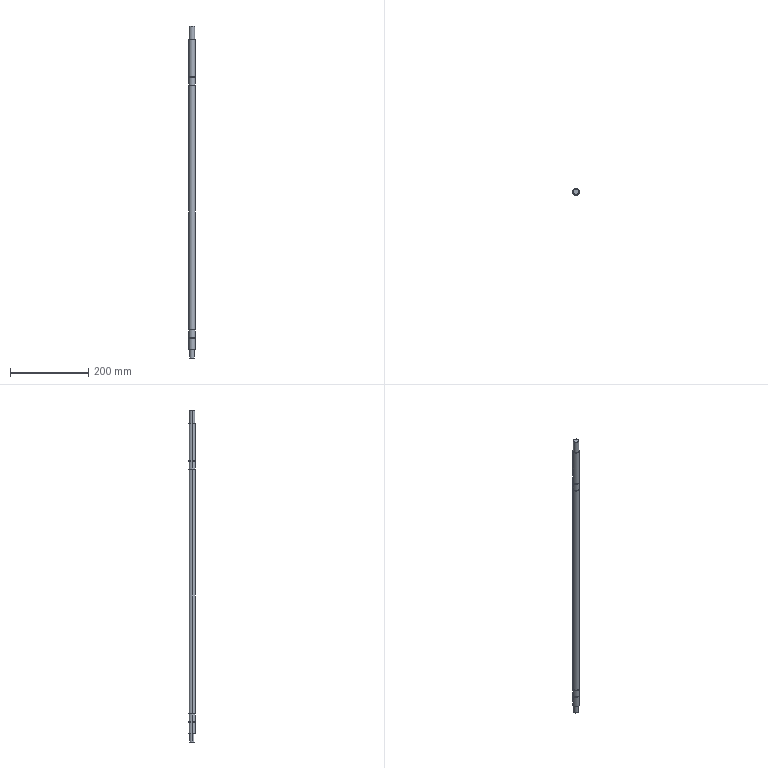Part | SolidWorks | features ICE 7, Cut 1, Extrusion 1, HoleWzd 1, MoveFace 1 | 1 solid | 42 faces | box 17 x 17 x 847.55 mm | volume 187223 mm3 | cylinder 25 | plane 15 | cone 2 | commonest cylinder face diameters 17 x10 16.2 x8 3.3 x2 12 x2 14 x2 4 x1
STEP:
#1=CARTESIAN_POINT('',(8.5,0.,-346.9));
#2=VERTEX_POINT('',#1);
#3=CARTESIAN_POINT('',(-8.5,0.,-346.9));
#4=VERTEX_POINT('',#3);
#5=CARTESIAN_POINT('',(0.,0.,-346.9));
#6=DIRECTION('',(0.,0.,1.));
#7=DIRECTION('',(1.,0.,0.));
#8=AXIS2_PLACEMENT_3D('',#5,#6,#7);
#9=CIRCLE('',#8,8.5);
#10=EDGE_CURVE('',#2,#4,#9,.T.);
#11=ORIENTED_EDGE('',*,*,#10,.F.);
#12=CARTESIAN_POINT('',(8.5,0.,-376.8));
#13=VERTEX_POINT('',#12);
#14=CARTESIAN_POINT('',(8.5,0.,416.8));
#15=DIRECTION('',(0.,0.,-1.));
#16=VECTOR('',#15,1000.);
#17=LINE('',#14,#16);
#18=EDGE_CURVE('',#2,#13,#17,.T.);
#19=ORIENTED_EDGE('',*,*,#18,.T.);
#20=CARTESIAN_POINT('',(-8.5,0.,-376.8));
#21=VERTEX_POINT('',#20);
#22=CARTESIAN_POINT('',(0.,0.,-376.8));
#23=DIRECTION('',(0.,0.,1.));
#24=DIRECTION('',(1.,0.,0.));
#25=AXIS2_PLACEMENT_3D('',#22,#23,#24);
#26=CIRCLE('',#25,8.5);
#27=EDGE_CURVE('',#13,#21,#26,.T.);
#28=ORIENTED_EDGE('',*,*,#27,.T.);
#29=CARTESIAN_POINT('',(-8.5,0.,416.8));
#30=DIRECTION('',(0.,0.,-1.));
#31=VECTOR('',#30,1000.);
#32=LINE('',#29,#31);
#33=EDGE_CURVE('',#4,#21,#32,.T.);
#34=ORIENTED_EDGE('',*,*,#33,.F.);
#35=EDGE_LOOP('',(#11,#19,#28,#34));
#36=FACE_OUTER_BOUND('',#35,.T.);
#37=CARTESIAN_POINT('',(0.,0.,416.8));
#38=DIRECTION('',(0.,0.,-1.));
#39=DIRECTION('',(-1.,0.,0.));
#40=AXIS2_PLACEMENT_3D('',#37,#38,#39);
#41=CYLINDRICAL_SURFACE('',#40,8.5);
#42=ADVANCED_FACE('',(#36),#41,.T.);
#43=CARTESIAN_POINT('',(-6.,0.,-376.8));
#44=VERTEX_POINT('',#43);
#45=CARTESIAN_POINT('',(6.,0.,-376.8));
#46=VERTEX_POINT('',#45);
#47=CARTESIAN_POINT('',(0.,0.,-376.8));
#48=DIRECTION('',(0.,0.,-1.));
#49=DIRECTION('',(1.,0.,0.));
#50=AXIS2_PLACEMENT_3D('',#47,#48,#49);
#51=CIRCLE('',#50,6.);
#52=EDGE_CURVE('',#44,#46,#51,.T.);
#53=ORIENTED_EDGE('',*,*,#52,.T.);
#54=CARTESIAN_POINT('',(6.,0.,-397.55));
#55=VERTEX_POINT('',#54);
#56=CARTESIAN_POINT('',(6.,0.,-392.758));
#57=DIRECTION('',(0.,0.,-1.));
#58=VECTOR('',#57,1000.);
#59=LINE('',#56,#58);
#60=EDGE_CURVE('',#46,#55,#59,.T.);
#61=ORIENTED_EDGE('',*,*,#60,.T.);
#62=CARTESIAN_POINT('',(2.,5.657,-397.55));
#63=VERTEX_POINT('',#62);
#64=CARTESIAN_POINT('',(0.,0.,-397.55));
#65=DIRECTION('',(0.,0.,-1.));
#66=DIRECTION('',(1.,0.,0.));
#67=AXIS2_PLACEMENT_3D('',#64,#65,#66);
#68=CIRCLE('',#67,6.);
#69=EDGE_CURVE('',#63,#55,#68,.T.);
#70=ORIENTED_EDGE('',*,*,#69,.F.);
#71=CARTESIAN_POINT('',(2.,5.657,-379.8));
#72=VERTEX_POINT('',#71);
#73=CARTESIAN_POINT('',(2.,5.657,-392.758));
#74=DIRECTION('',(0.,0.,-1.));
#75=VECTOR('',#74,1000.);
#76=LINE('',#73,#75);
#77=EDGE_CURVE('',#72,#63,#76,.T.);
#78=ORIENTED_EDGE('',*,*,#77,.F.);
#79=CARTESIAN_POINT('',(-2.,5.657,-379.8));
#80=VERTEX_POINT('',#79);
#81=CARTESIAN_POINT('',(-2.,5.657,-379.8));
#82=CARTESIAN_POINT('',(-2.,5.657,-379.667));
#83=CARTESIAN_POINT('',(-1.987,5.662,-379.536));
#84=CARTESIAN_POINT('',(-1.935,5.679,-379.279));
#85=CARTESIAN_POINT('',(-1.897,5.693,-379.152));
#86=CARTESIAN_POINT('',(-1.796,5.725,-378.91));
#87=CARTESIAN_POINT('',(-1.735,5.744,-378.796));
#88=CARTESIAN_POINT('',(-1.59,5.786,-378.579));
#89=CARTESIAN_POINT('',(-1.506,5.809,-378.477));
#90=CARTESIAN_POINT('',(-1.231,5.875,-378.203));
#91=CARTESIAN_POINT('',(-1.01,5.919,-378.054));
#92=CARTESIAN_POINT('',(-0.6496,5.966,-377.904));
#93=CARTESIAN_POINT('',(-0.5226,5.979,-377.865));
#94=CARTESIAN_POINT('',(-0.264,5.996,-377.813));
#95=CARTESIAN_POINT('',(-0.1336,6.,-377.8));
#96=CARTESIAN_POINT('',(0.1294,6.,-377.8));
#97=CARTESIAN_POINT('',(0.2629,5.996,-377.813));
#98=CARTESIAN_POINT('',(0.5202,5.979,-377.864));
#99=CARTESIAN_POINT('',(0.6454,5.966,-377.902));
#100=CARTESIAN_POINT('',(0.8889,5.935,-378.004));
#101=CARTESIAN_POINT('',(1.004,5.916,-378.066));
#102=CARTESIAN_POINT('',(1.22,5.876,-378.21));
#103=CARTESIAN_POINT('',(1.322,5.853,-378.293));
#104=CARTESIAN_POINT('',(1.506,5.809,-378.477));
#105=CARTESIAN_POINT('',(1.588,5.787,-378.577));
#106=CARTESIAN_POINT('',(1.733,5.745,-378.793));
#107=CARTESIAN_POINT('',(1.796,5.725,-378.91));
#108=CARTESIAN_POINT('',(1.946,5.677,-379.271));
#109=CARTESIAN_POINT('',(2.,5.657,-379.534));
#110=CARTESIAN_POINT('',(2.,5.657,-379.8));
#111=B_SPLINE_CURVE_WITH_KNOTS('',3,(#81,#82,#83,#84,#85,#86,#87,#88,#89,#90,#91,#92,#93,#94,#95,#96,#97,#98,#99,#100,#101,#102,#103,#104,#105,#106,#107,#108,#109,#110),.UNSPECIFIED.,.F.,.F.,(4,2,2,2,2,2,2,2,2,2,2,2,2,2,4),(0.,0.0003935,0.000787,0.00118,0.001574,0.002361,0.002754,0.003148,0.003541,0.003935,0.004328,0.004722,0.005115,0.005509,0.006296),.UNSPECIFIED.);
#112=EDGE_CURVE('',#80,#72,#111,.T.);
#113=ORIENTED_EDGE('',*,*,#112,.F.);
#114=CARTESIAN_POINT('',(-2.,5.657,-397.55));
#115=VERTEX_POINT('',#114);
#116=CARTESIAN_POINT('',(-2.,5.657,-392.758));
#117=DIRECTION('',(0.,0.,1.));
#118=VECTOR('',#117,1000.);
#119=LINE('',#116,#118);
#120=EDGE_CURVE('',#115,#80,#119,.T.);
#121=ORIENTED_EDGE('',*,*,#120,.F.);
#122=CARTESIAN_POINT('',(-6.,0.,-397.55));
#123=VERTEX_POINT('',#122);
#124=CARTESIAN_POINT('',(0.,0.,-397.55));
#125=DIRECTION('',(0.,0.,-1.));
#126=DIRECTION('',(1.,0.,0.));
#127=AXIS2_PLACEMENT_3D('',#124,#125,#126);
#128=CIRCLE('',#127,6.);
#129=EDGE_CURVE('',#123,#115,#128,.T.);
#130=ORIENTED_EDGE('',*,*,#129,.F.);
#131=CARTESIAN_POINT('',(-6.,0.,-392.758));
#132=DIRECTION('',(0.,0.,-1.));
#133=VECTOR('',#132,1000.);
#134=LINE('',#131,#133);
#135=EDGE_CURVE('',#44,#123,#134,.T.);
#136=ORIENTED_EDGE('',*,*,#135,.F.);
#137=EDGE_LOOP('',(#53,#61,#70,#78,#113,#121,#130,#136));
#138=FACE_OUTER_BOUND('',#137,.T.);
#139=CARTESIAN_POINT('',(0.,0.,-392.758));
#140=DIRECTION('',(0.,0.,-1.));
#141=DIRECTION('',(-1.,0.,0.));
#142=AXIS2_PLACEMENT_3D('',#139,#140,#141);
#143=CYLINDRICAL_SURFACE('',#142,6.);
#144=ADVANCED_FACE('',(#138),#143,.T.);
#145=CARTESIAN_POINT('',(1.65,0.,-387.45));
#146=VERTEX_POINT('',#145);
#147=CARTESIAN_POINT('',(-1.65,0.,-387.45));
#148=VERTEX_POINT('',#147);
#149=CARTESIAN_POINT('',(0.,0.,-387.45));
#150=DIRECTION('',(0.,0.,-1.));
#151=DIRECTION('',(-1.,0.,0.));
#152=AXIS2_PLACEMENT_3D('',#149,#150,#151);
#153=CIRCLE('',#152,1.65);
#154=EDGE_CURVE('',#146,#148,#153,.T.);
#155=ORIENTED_EDGE('',*,*,#154,.F.);
#156=CARTESIAN_POINT('',(1.65,0.,-397.55));
#157=VERTEX_POINT('',#156);
#158=CARTESIAN_POINT('',(1.65,0.,-397.55));
#159=DIRECTION('',(0.,0.,-1.));
#160=VECTOR('',#159,1000.);
#161=LINE('',#158,#160);
#162=EDGE_CURVE('',#146,#157,#161,.T.);
#163=ORIENTED_EDGE('',*,*,#162,.T.);
#164=CARTESIAN_POINT('',(-1.65,0.,-397.55));
#165=VERTEX_POINT('',#164);
#166=CARTESIAN_POINT('',(0.,0.,-397.55));
#167=DIRECTION('',(0.,0.,-1.));
#168=DIRECTION('',(-1.,0.,0.));
#169=AXIS2_PLACEMENT_3D('',#166,#167,#168);
#170=CIRCLE('',#169,1.65);
#171=EDGE_CURVE('',#157,#165,#170,.T.);
#172=ORIENTED_EDGE('',*,*,#171,.T.);
#173=CARTESIAN_POINT('',(-1.65,0.,-397.55));
#174=DIRECTION('',(0.,0.,-1.));
#175=VECTOR('',#174,1000.);
#176=LINE('',#173,#175);
#177=EDGE_CURVE('',#148,#165,#176,.T.);
#178=ORIENTED_EDGE('',*,*,#177,.F.);
#179=EDGE_LOOP('',(#155,#163,#172,#178));
#180=FACE_OUTER_BOUND('',#179,.T.);
#181=CARTESIAN_POINT('',(0.,0.,-397.55));
#182=DIRECTION('',(0.,0.,-1.));
#183=DIRECTION('',(-1.,0.,0.));
#184=AXIS2_PLACEMENT_3D('',#181,#182,#183);
#185=CYLINDRICAL_SURFACE('',#184,1.65);
#186=ADVANCED_FACE('',(#180),#185,.F.);
#187=CARTESIAN_POINT('',(0.,0.,-386.459));
#188=VERTEX_POINT('',#187);
#189=CARTESIAN_POINT('',(-1.65,0.,-387.45));
#190=DIRECTION('',(-0.8572,0.,-0.515));
#191=VECTOR('',#190,1000.);
#192=LINE('',#189,#191);
#193=EDGE_CURVE('',#188,#148,#192,.T.);
#194=ORIENTED_EDGE('',*,*,#193,.F.);
#195=CARTESIAN_POINT('',(1.65,0.,-387.45));
#196=DIRECTION('',(0.8572,0.,-0.515));
#197=VECTOR('',#196,1000.);
#198=LINE('',#195,#197);
#199=EDGE_CURVE('',#188,#146,#198,.T.);
#200=ORIENTED_EDGE('',*,*,#199,.T.);
#201=ORIENTED_EDGE('',*,*,#154,.T.);
#202=EDGE_LOOP('',(#194,#200,#201));
#203=FACE_OUTER_BOUND('',#202,.T.);
#204=CARTESIAN_POINT('',(0.,0.,-387.45));
#205=DIRECTION('',(0.,0.,-1.));
#206=DIRECTION('',(-1.,0.,0.));
#207=AXIS2_PLACEMENT_3D('',#204,#205,#206);
#208=CONICAL_SURFACE('',#207,1.65,1.03);
#209=ADVANCED_FACE('',(#203),#208,.F.);
#210=CARTESIAN_POINT('',(8.1,0.,-345.8));
#211=VERTEX_POINT('',#210);
#212=CARTESIAN_POINT('',(-8.1,0.,-345.8));
#213=VERTEX_POINT('',#212);
#214=CARTESIAN_POINT('',(0.,0.,-345.8));
#215=DIRECTION('',(0.,0.,1.));
#216=DIRECTION('',(1.,0.,0.));
#217=AXIS2_PLACEMENT_3D('',#214,#215,#216);
#218=CIRCLE('',#217,8.1);
#219=EDGE_CURVE('',#211,#213,#218,.T.);
#220=ORIENTED_EDGE('',*,*,#219,.F.);
#221=CARTESIAN_POINT('',(8.1,0.,-346.9));
#222=VERTEX_POINT('',#221);
#223=CARTESIAN_POINT('',(8.1,0.,-345.8));
#224=DIRECTION('',(0.,0.,-1.));
#225=VECTOR('',#224,1000.);
#226=LINE('',#223,#225);
#227=EDGE_CURVE('',#211,#222,#226,.T.);
#228=ORIENTED_EDGE('',*,*,#227,.T.);
#229=CARTESIAN_POINT('',(-8.1,0.,-346.9));
#230=VERTEX_POINT('',#229);
#231=CARTESIAN_POINT('',(0.,0.,-346.9));
#232=DIRECTION('',(0.,0.,1.));
#233=DIRECTION('',(1.,0.,0.));
#234=AXIS2_PLACEMENT_3D('',#231,#232,#233);
#235=CIRCLE('',#234,8.1);
#236=EDGE_CURVE('',#222,#230,#235,.T.);
#237=ORIENTED_EDGE('',*,*,#236,.T.);
#238=CARTESIAN_POINT('',(-8.1,0.,-345.8));
#239=DIRECTION('',(0.,0.,-1.));
#240=VECTOR('',#239,1000.);
#241=LINE('',#238,#240);
#242=EDGE_CURVE('',#213,#230,#241,.T.);
#243=ORIENTED_EDGE('',*,*,#242,.F.);
#244=EDGE_LOOP('',(#220,#228,#237,#243));
#245=FACE_OUTER_BOUND('',#244,.T.);
#246=CARTESIAN_POINT('',(0.,0.,-345.8));
#247=DIRECTION('',(0.,0.,-1.));
#248=DIRECTION('',(-1.,0.,0.));
#249=AXIS2_PLACEMENT_3D('',#246,#247,#248);
#250=CYLINDRICAL_SURFACE('',#249,8.1);
#251=ADVANCED_FACE('',(#245),#250,.T.);
#252=CARTESIAN_POINT('',(8.5,0.,-325.8));
#253=VERTEX_POINT('',#252);
#254=CARTESIAN_POINT('',(-8.5,0.,-325.8));
#255=VERTEX_POINT('',#254);
#256=CARTESIAN_POINT('',(0.,0.,-325.8));
#257=DIRECTION('',(0.,0.,1.));
#258=DIRECTION('',(1.,0.,0.));
#259=AXIS2_PLACEMENT_3D('',#256,#257,#258);
#260=CIRCLE('',#259,8.5);
#261=EDGE_CURVE('',#253,#255,#260,.T.);
#262=ORIENTED_EDGE('',*,*,#261,.F.);
#263=CARTESIAN_POINT('',(8.5,0.,-345.8));
#264=VERTEX_POINT('',#263);
#265=CARTESIAN_POINT('',(8.5,0.,416.8));
#266=DIRECTION('',(0.,0.,-1.));
#267=VECTOR('',#266,1000.);
#268=LINE('',#265,#267);
#269=EDGE_CURVE('',#253,#264,#268,.T.);
#270=ORIENTED_EDGE('',*,*,#269,.T.);
#271=CARTESIAN_POINT('',(-8.5,0.,-345.8));
#272=VERTEX_POINT('',#271);
#273=CARTESIAN_POINT('',(0.,0.,-345.8));
#274=DIRECTION('',(0.,0.,1.));
#275=DIRECTION('',(1.,0.,0.));
#276=AXIS2_PLACEMENT_3D('',#273,#274,#275);
#277=CIRCLE('',#276,8.5);
#278=EDGE_CURVE('',#264,#272,#277,.T.);
#279=ORIENTED_EDGE('',*,*,#278,.T.);
#280=CARTESIAN_POINT('',(-8.5,0.,416.8));
#281=DIRECTION('',(0.,0.,-1.));
#282=VECTOR('',#281,1000.);
#283=LINE('',#280,#282);
#284=EDGE_CURVE('',#255,#272,#283,.T.);
#285=ORIENTED_EDGE('',*,*,#284,.F.);
#286=EDGE_LOOP('',(#262,#270,#279,#285));
#287=FACE_OUTER_BOUND('',#286,.T.);
#288=CARTESIAN_POINT('',(0.,0.,416.8));
#289=DIRECTION('',(0.,0.,-1.));
#290=DIRECTION('',(-1.,0.,0.));
#291=AXIS2_PLACEMENT_3D('',#288,#289,#290);
#292=CYLINDRICAL_SURFACE('',#291,8.5);
#293=ADVANCED_FACE('',(#287),#292,.T.);
#294=CARTESIAN_POINT('',(8.1,0.,-324.7));
#295=VERTEX_POINT('',#294);
#296=CARTESIAN_POINT('',(-8.1,0.,-324.7));
#297=VERTEX_POINT('',#296);
#298=CARTESIAN_POINT('',(0.,0.,-324.7));
#299=DIRECTION('',(0.,0.,1.));
#300=DIRECTION('',(1.,0.,0.));
#301=AXIS2_PLACEMENT_3D('',#298,#299,#300);
#302=CIRCLE('',#301,8.1);
#303=EDGE_CURVE('',#295,#297,#302,.T.);
#304=ORIENTED_EDGE('',*,*,#303,.F.);
#305=CARTESIAN_POINT('',(8.1,0.,-325.8));
#306=VERTEX_POINT('',#305);
#307=CARTESIAN_POINT('',(8.1,0.,-324.7));
#308=DIRECTION('',(0.,0.,-1.));
#309=VECTOR('',#308,1000.);
#310=LINE('',#307,#309);
#311=EDGE_CURVE('',#295,#306,#310,.T.);
#312=ORIENTED_EDGE('',*,*,#311,.T.);
#313=CARTESIAN_POINT('',(-8.1,0.,-325.8));
#314=VERTEX_POINT('',#313);
#315=CARTESIAN_POINT('',(0.,0.,-325.8));
#316=DIRECTION('',(0.,0.,1.));
#317=DIRECTION('',(1.,0.,0.));
#318=AXIS2_PLACEMENT_3D('',#315,#316,#317);
#319=CIRCLE('',#318,8.1);
#320=EDGE_CURVE('',#306,#314,#319,.T.);
#321=ORIENTED_EDGE('',*,*,#320,.T.);
#322=CARTESIAN_POINT('',(-8.1,0.,-324.7));
#323=DIRECTION('',(0.,0.,-1.));
#324=VECTOR('',#323,1000.);
#325=LINE('',#322,#324);
#326=EDGE_CURVE('',#297,#314,#325,.T.);
#327=ORIENTED_EDGE('',*,*,#326,.F.);
#328=EDGE_LOOP('',(#304,#312,#321,#327));
#329=FACE_OUTER_BOUND('',#328,.T.);
#330=CARTESIAN_POINT('',(0.,0.,-324.7));
#331=DIRECTION('',(0.,0.,-1.));
#332=DIRECTION('',(-1.,0.,0.));
#333=AXIS2_PLACEMENT_3D('',#330,#331,#332);
#334=CYLINDRICAL_SURFACE('',#333,8.1);
#335=ADVANCED_FACE('',(#329),#334,.T.);
#336=CARTESIAN_POINT('',(8.5,0.,298.1));
#337=VERTEX_POINT('',#336);
#338=CARTESIAN_POINT('',(-8.5,0.,298.1));
#339=VERTEX_POINT('',#338);
#340=CARTESIAN_POINT('',(0.,0.,298.1));
#341=DIRECTION('',(0.,0.,1.));
#342=DIRECTION('',(1.,0.,0.));
#343=AXIS2_PLACEMENT_3D('',#340,#341,#342);
#344=CIRCLE('',#343,8.5);
#345=EDGE_CURVE('',#337,#339,#344,.T.);
#346=ORIENTED_EDGE('',*,*,#345,.F.);
#347=CARTESIAN_POINT('',(8.5,0.,-324.7));
#348=VERTEX_POINT('',#347);
#349=CARTESIAN_POINT('',(8.5,0.,416.8));
#350=DIRECTION('',(0.,0.,-1.));
#351=VECTOR('',#350,1000.);
#352=LINE('',#349,#351);
#353=EDGE_CURVE('',#337,#348,#352,.T.);
#354=ORIENTED_EDGE('',*,*,#353,.T.);
#355=CARTESIAN_POINT('',(-8.5,0.,-324.7));
#356=VERTEX_POINT('',#355);
#357=CARTESIAN_POINT('',(0.,0.,-324.7));
#358=DIRECTION('',(0.,0.,1.));
#359=DIRECTION('',(1.,0.,0.));
#360=AXIS2_PLACEMENT_3D('',#357,#358,#359);
#361=CIRCLE('',#360,8.5);
#362=EDGE_CURVE('',#348,#356,#361,.T.);
#363=ORIENTED_EDGE('',*,*,#362,.T.);
#364=CARTESIAN_POINT('',(-8.5,0.,416.8));
#365=DIRECTION('',(0.,0.,-1.));
#366=VECTOR('',#365,1000.);
#367=LINE('',#364,#366);
#368=EDGE_CURVE('',#339,#356,#367,.T.);
#369=ORIENTED_EDGE('',*,*,#368,.F.);
#370=EDGE_LOOP('',(#346,#354,#363,#369));
#371=FACE_OUTER_BOUND('',#370,.T.);
#372=CARTESIAN_POINT('',(0.,0.,416.8));
#373=DIRECTION('',(0.,0.,-1.));
#374=DIRECTION('',(-1.,0.,0.));
#375=AXIS2_PLACEMENT_3D('',#372,#373,#374);
#376=CYLINDRICAL_SURFACE('',#375,8.5);
#377=ADVANCED_FACE('',(#371),#376,.T.);
#378=CARTESIAN_POINT('',(8.1,0.,299.2));
#379=VERTEX_POINT('',#378);
#380=CARTESIAN_POINT('',(-8.1,0.,299.2));
#381=VERTEX_POINT('',#380);
#382=CARTESIAN_POINT('',(0.,0.,299.2));
#383=DIRECTION('',(0.,0.,1.));
#384=DIRECTION('',(1.,0.,0.));
#385=AXIS2_PLACEMENT_3D('',#382,#383,#384);
#386=CIRCLE('',#385,8.1);
#387=EDGE_CURVE('',#379,#381,#386,.T.);
#388=ORIENTED_EDGE('',*,*,#387,.F.);
#389=CARTESIAN_POINT('',(8.1,0.,298.1));
#390=VERTEX_POINT('',#389);
#391=CARTESIAN_POINT('',(8.1,0.,299.2));
#392=DIRECTION('',(0.,0.,-1.));
#393=VECTOR('',#392,1000.);
#394=LINE('',#391,#393);
#395=EDGE_CURVE('',#379,#390,#394,.T.);
#396=ORIENTED_EDGE('',*,*,#395,.T.);
#397=CARTESIAN_POINT('',(-8.1,0.,298.1));
#398=VERTEX_POINT('',#397);
#399=CARTESIAN_POINT('',(0.,0.,298.1));
#400=DIRECTION('',(0.,0.,1.));
#401=DIRECTION('',(1.,0.,0.));
#402=AXIS2_PLACEMENT_3D('',#399,#400,#401);
#403=CIRCLE('',#402,8.1);
#404=EDGE_CURVE('',#390,#398,#403,.T.);
#405=ORIENTED_EDGE('',*,*,#404,.T.);
#406=CARTESIAN_POINT('',(-8.1,0.,299.2));
#407=DIRECTION('',(0.,0.,-1.));
#408=VECTOR('',#407,1000.);
#409=LINE('',#406,#408);
#410=EDGE_CURVE('',#381,#398,#409,.T.);
#411=ORIENTED_EDGE('',*,*,#410,.F.);
#412=EDGE_LOOP('',(#388,#396,#405,#411));
#413=FACE_OUTER_BOUND('',#412,.T.);
#414=CARTESIAN_POINT('',(0.,0.,299.2));
#415=DIRECTION('',(0.,0.,-1.));
#416=DIRECTION('',(-1.,0.,0.));
#417=AXIS2_PLACEMENT_3D('',#414,#415,#416);
#418=CYLINDRICAL_SURFACE('',#417,8.1);
#419=ADVANCED_FACE('',(#413),#418,.T.);
#420=CARTESIAN_POINT('',(8.5,0.,416.8));
#421=VERTEX_POINT('',#420);
#422=CARTESIAN_POINT('',(-8.5,0.,416.8));
#423=VERTEX_POINT('',#422);
#424=CARTESIAN_POINT('',(0.,0.,416.8));
#425=DIRECTION('',(0.,0.,1.));
#426=DIRECTION('',(1.,0.,0.));
#427=AXIS2_PLACEMENT_3D('',#424,#425,#426);
#428=CIRCLE('',#427,8.5);
#429=EDGE_CURVE('',#421,#423,#428,.T.);
#430=ORIENTED_EDGE('',*,*,#429,.F.);
#431=CARTESIAN_POINT('',(8.5,0.,320.3));
#432=VERTEX_POINT('',#431);
#433=CARTESIAN_POINT('',(8.5,0.,416.8));
#434=DIRECTION('',(0.,0.,-1.));
#435=VECTOR('',#434,1000.);
#436=LINE('',#433,#435);
#437=EDGE_CURVE('',#421,#432,#436,.T.);
#438=ORIENTED_EDGE('',*,*,#437,.T.);
#439=CARTESIAN_POINT('',(-8.5,0.,320.3));
#440=VERTEX_POINT('',#439);
#441=CARTESIAN_POINT('',(0.,0.,320.3));
#442=DIRECTION('',(0.,0.,1.));
#443=DIRECTION('',(1.,0.,0.));
#444=AXIS2_PLACEMENT_3D('',#441,#442,#443);
#445=CIRCLE('',#444,8.5);
#446=EDGE_CURVE('',#432,#440,#445,.T.);
#447=ORIENTED_EDGE('',*,*,#446,.T.);
#448=CARTESIAN_POINT('',(-8.5,0.,416.8));
#449=DIRECTION('',(0.,0.,-1.));
#450=VECTOR('',#449,1000.);
#451=LINE('',#448,#450);
#452=EDGE_CURVE('',#423,#440,#451,.T.);
#453=ORIENTED_EDGE('',*,*,#452,.F.);
#454=EDGE_LOOP('',(#430,#438,#447,#453));
#455=FACE_OUTER_BOUND('',#454,.T.);
#456=CARTESIAN_POINT('',(0.,0.,416.8));
#457=DIRECTION('',(0.,0.,-1.));
#458=DIRECTION('',(-1.,0.,0.));
#459=AXIS2_PLACEMENT_3D('',#456,#457,#458);
#460=CYLINDRICAL_SURFACE('',#459,8.5);
#461=ADVANCED_FACE('',(#455),#460,.T.);
#462=CARTESIAN_POINT('',(7.,0.,450.));
#463=VERTEX_POINT('',#462);
#464=CARTESIAN_POINT('',(-7.,0.,450.));
#465=VERTEX_POINT('',#464);
#466=CARTESIAN_POINT('',(0.,0.,450.));
#467=DIRECTION('',(0.,0.,1.));
#468=DIRECTION('',(1.,0.,0.));
#469=AXIS2_PLACEMENT_3D('',#466,#467,#468);
#470=CIRCLE('',#469,7.);
#471=EDGE_CURVE('',#463,#465,#470,.T.);
#472=ORIENTED_EDGE('',*,*,#471,.F.);
#473=CARTESIAN_POINT('',(7.,0.,416.8));
#474=VERTEX_POINT('',#473);
#475=CARTESIAN_POINT('',(7.,0.,450.));
#476=DIRECTION('',(0.,0.,-1.));
#477=VECTOR('',#476,1000.);
#478=LINE('',#475,#477);
#479=EDGE_CURVE('',#463,#474,#478,.T.);
#480=ORIENTED_EDGE('',*,*,#479,.T.);
#481=CARTESIAN_POINT('',(-7.,0.,416.8));
#482=VERTEX_POINT('',#481);
#483=CARTESIAN_POINT('',(0.,0.,416.8));
#484=DIRECTION('',(0.,0.,1.));
#485=DIRECTION('',(1.,0.,0.));
#486=AXIS2_PLACEMENT_3D('',#483,#484,#485);
#487=CIRCLE('',#486,7.);
#488=EDGE_CURVE('',#474,#482,#487,.T.);
#489=ORIENTED_EDGE('',*,*,#488,.T.);
#490=CARTESIAN_POINT('',(-7.,0.,450.));
#491=DIRECTION('',(0.,0.,-1.));
#492=VECTOR('',#491,1000.);
#493=LINE('',#490,#492);
#494=EDGE_CURVE('',#465,#482,#493,.T.);
#495=ORIENTED_EDGE('',*,*,#494,.F.);
#496=EDGE_LOOP('',(#472,#480,#489,#495));
#497=FACE_OUTER_BOUND('',#496,.T.);
#498=CARTESIAN_POINT('',(0.,0.,450.));
#499=DIRECTION('',(0.,0.,-1.));
#500=DIRECTION('',(-1.,0.,0.));
#501=AXIS2_PLACEMENT_3D('',#498,#499,#500);
#502=CYLINDRICAL_SURFACE('',#501,7.);
#503=ADVANCED_FACE('',(#497),#502,.T.);
#504=CARTESIAN_POINT('',(8.1,0.,320.3));
#505=VERTEX_POINT('',#504);
#506=CARTESIAN_POINT('',(-8.1,0.,320.3));
#507=VERTEX_POINT('',#506);
#508=CARTESIAN_POINT('',(0.,0.,320.3));
#509=DIRECTION('',(0.,0.,1.));
#510=DIRECTION('',(1.,0.,0.));
#511=AXIS2_PLACEMENT_3D('',#508,#509,#510);
#512=CIRCLE('',#511,8.1);
#513=EDGE_CURVE('',#505,#507,#512,.T.);
#514=ORIENTED_EDGE('',*,*,#513,.F.);
#515=CARTESIAN_POINT('',(8.1,0.,319.2));
#516=VERTEX_POINT('',#515);
#517=CARTESIAN_POINT('',(8.1,0.,320.3));
#518=DIRECTION('',(0.,0.,-1.));
#519=VECTOR('',#518,1000.);
#520=LINE('',#517,#519);
#521=EDGE_CURVE('',#505,#516,#520,.T.);
#522=ORIENTED_EDGE('',*,*,#521,.T.);
#523=CARTESIAN_POINT('',(-8.1,0.,319.2));
#524=VERTEX_POINT('',#523);
#525=CARTESIAN_POINT('',(0.,0.,319.2));
#526=DIRECTION('',(0.,0.,1.));
#527=DIRECTION('',(1.,0.,0.));
#528=AXIS2_PLACEMENT_3D('',#525,#526,#527);
#529=CIRCLE('',#528,8.1);
#530=EDGE_CURVE('',#516,#524,#529,.T.);
#531=ORIENTED_EDGE('',*,*,#530,.T.);
#532=CARTESIAN_POINT('',(-8.1,0.,320.3));
#533=DIRECTION('',(0.,0.,-1.));
#534=VECTOR('',#533,1000.);
#535=LINE('',#532,#534);
#536=EDGE_CURVE('',#507,#524,#535,.T.);
#537=ORIENTED_EDGE('',*,*,#536,.F.);
#538=EDGE_LOOP('',(#514,#522,#531,#537));
#539=FACE_OUTER_BOUND('',#538,.T.);
#540=CARTESIAN_POINT('',(0.,0.,320.3));
#541=DIRECTION('',(0.,0.,-1.));
#542=DIRECTION('',(-1.,0.,0.));
#543=AXIS2_PLACEMENT_3D('',#540,#541,#542);
#544=CYLINDRICAL_SURFACE('',#543,8.1);
#545=ADVANCED_FACE('',(#539),#544,.T.);
#546=CARTESIAN_POINT('',(8.5,0.,319.2));
#547=VERTEX_POINT('',#546);
#548=CARTESIAN_POINT('',(-8.5,0.,319.2));
#549=VERTEX_POINT('',#548);
#550=CARTESIAN_POINT('',(0.,0.,319.2));
#551=DIRECTION('',(0.,0.,1.));
#552=DIRECTION('',(1.,0.,0.));
#553=AXIS2_PLACEMENT_3D('',#550,#551,#552);
#554=CIRCLE('',#553,8.5);
#555=EDGE_CURVE('',#547,#549,#554,.T.);
#556=ORIENTED_EDGE('',*,*,#555,.F.);
#557=CARTESIAN_POINT('',(8.5,0.,299.2));
#558=VERTEX_POINT('',#557);
#559=CARTESIAN_POINT('',(8.5,0.,416.8));
#560=DIRECTION('',(0.,0.,-1.));
#561=VECTOR('',#560,1000.);
#562=LINE('',#559,#561);
#563=EDGE_CURVE('',#547,#558,#562,.T.);
#564=ORIENTED_EDGE('',*,*,#563,.T.);
#565=CARTESIAN_POINT('',(-8.5,0.,299.2));
#566=VERTEX_POINT('',#565);
#567=CARTESIAN_POINT('',(0.,0.,299.2));
#568=DIRECTION('',(0.,0.,1.));
#569=DIRECTION('',(1.,0.,0.));
#570=AXIS2_PLACEMENT_3D('',#567,#568,#569);
#571=CIRCLE('',#570,8.5);
#572=EDGE_CURVE('',#558,#566,#571,.T.);
#573=ORIENTED_EDGE('',*,*,#572,.T.);
#574=CARTESIAN_POINT('',(-8.5,0.,416.8));
#575=DIRECTION('',(0.,0.,-1.));
#576=VECTOR('',#575,1000.);
#577=LINE('',#574,#576);
#578=EDGE_CURVE('',#549,#566,#577,.T.);
#579=ORIENTED_EDGE('',*,*,#578,.F.);
#580=EDGE_LOOP('',(#556,#564,#573,#579));
#581=FACE_OUTER_BOUND('',#580,.T.);
#582=CARTESIAN_POINT('',(0.,0.,416.8));
#583=DIRECTION('',(0.,0.,-1.));
#584=DIRECTION('',(-1.,0.,0.));
#585=AXIS2_PLACEMENT_3D('',#582,#583,#584);
#586=CYLINDRICAL_SURFACE('',#585,8.5);
#587=ADVANCED_FACE('',(#581),#586,.T.);
#588=ORIENTED_EDGE('',*,*,#563,.F.);
#589=CARTESIAN_POINT('',(0.,0.,319.2));
#590=DIRECTION('',(0.,0.,1.));
#591=DIRECTION('',(1.,0.,0.));
#592=AXIS2_PLACEMENT_3D('',#589,#590,#591);
#593=CIRCLE('',#592,8.5);
#594=EDGE_CURVE('',#549,#547,#593,.T.);
#595=ORIENTED_EDGE('',*,*,#594,.F.);
#596=ORIENTED_EDGE('',*,*,#578,.T.);
#597=CARTESIAN_POINT('',(0.,0.,299.2));
#598=DIRECTION('',(0.,0.,1.));
#599=DIRECTION('',(1.,0.,0.));
#600=AXIS2_PLACEMENT_3D('',#597,#598,#599);
#601=CIRCLE('',#600,8.5);
#602=EDGE_CURVE('',#566,#558,#601,.T.);
#603=ORIENTED_EDGE('',*,*,#602,.T.);
#604=EDGE_LOOP('',(#588,#595,#596,#603));
#605=FACE_OUTER_BOUND('',#604,.T.);
#606=CARTESIAN_POINT('',(0.,0.,416.8));
#607=DIRECTION('',(0.,0.,-1.));
#608=DIRECTION('',(-1.,0.,0.));
#609=AXIS2_PLACEMENT_3D('',#606,#607,#608);
#610=CYLINDRICAL_SURFACE('',#609,8.5);
#611=ADVANCED_FACE('',(#605),#610,.T.);
#612=CARTESIAN_POINT('',(0.,0.,320.3));
#613=DIRECTION('',(0.,0.,1.));
#614=DIRECTION('',(1.,0.,0.));
#615=AXIS2_PLACEMENT_3D('',#612,#613,#614);
#616=CIRCLE('',#615,8.5);
#617=EDGE_CURVE('',#440,#432,#616,.T.);
#618=ORIENTED_EDGE('',*,*,#617,.F.);
#619=ORIENTED_EDGE('',*,*,#446,.F.);
#620=EDGE_LOOP('',(#618,#619));
#621=FACE_OUTER_BOUND('',#620,.T.);
#622=CARTESIAN_POINT('',(0.,0.,320.3));
#623=DIRECTION('',(0.,0.,1.));
#624=DIRECTION('',(1.,0.,0.));
#625=AXIS2_PLACEMENT_3D('',#622,#623,#624);
#626=CIRCLE('',#625,8.1);
#627=EDGE_CURVE('',#507,#505,#626,.T.);
#628=ORIENTED_EDGE('',*,*,#627,.T.);
#629=ORIENTED_EDGE('',*,*,#513,.T.);
#630=EDGE_LOOP('',(#628,#629));
#631=FACE_BOUND('',#630,.T.);
#632=CARTESIAN_POINT('',(0.,0.,320.3));
#633=DIRECTION('',(0.,0.,1.));
#634=DIRECTION('',(1.,0.,0.));
#635=AXIS2_PLACEMENT_3D('',#632,#633,#634);
#636=PLANE('',#635);
#637=ADVANCED_FACE('',(#621,#631),#636,.F.);
#638=ORIENTED_EDGE('',*,*,#594,.T.);
#639=ORIENTED_EDGE('',*,*,#555,.T.);
#640=EDGE_LOOP('',(#638,#639));
#641=FACE_OUTER_BOUND('',#640,.T.);
#642=CARTESIAN_POINT('',(0.,0.,319.2));
#643=DIRECTION('',(0.,0.,1.));
#644=DIRECTION('',(1.,0.,0.));
#645=AXIS2_PLACEMENT_3D('',#642,#643,#644);
#646=CIRCLE('',#645,8.1);
#647=EDGE_CURVE('',#524,#516,#646,.T.);
#648=ORIENTED_EDGE('',*,*,#647,.F.);
#649=ORIENTED_EDGE('',*,*,#530,.F.);
#650=EDGE_LOOP('',(#648,#649));
#651=FACE_BOUND('',#650,.T.);
#652=CARTESIAN_POINT('',(0.,0.,319.2));
#653=DIRECTION('',(0.,0.,1.));
#654=DIRECTION('',(1.,0.,0.));
#655=AXIS2_PLACEMENT_3D('',#652,#653,#654);
#656=PLANE('',#655);
#657=ADVANCED_FACE('',(#641,#651),#656,.T.);
#658=ORIENTED_EDGE('',*,*,#521,.F.);
#659=ORIENTED_EDGE('',*,*,#627,.F.);
#660=ORIENTED_EDGE('',*,*,#536,.T.);
#661=ORIENTED_EDGE('',*,*,#647,.T.);
#662=EDGE_LOOP('',(#658,#659,#660,#661));
#663=FACE_OUTER_BOUND('',#662,.T.);
#664=CARTESIAN_POINT('',(0.,0.,320.3));
#665=DIRECTION('',(0.,0.,-1.));
#666=DIRECTION('',(-1.,0.,0.));
#667=AXIS2_PLACEMENT_3D('',#664,#665,#666);
#668=CYLINDRICAL_SURFACE('',#667,8.1);
#669=ADVANCED_FACE('',(#663),#668,.T.);
#670=CARTESIAN_POINT('',(0.,0.,450.));
#671=DIRECTION('',(0.,0.,1.));
#672=DIRECTION('',(1.,0.,0.));
#673=AXIS2_PLACEMENT_3D('',#670,#671,#672);
#674=CIRCLE('',#673,7.);
#675=EDGE_CURVE('',#465,#463,#674,.T.);
#676=ORIENTED_EDGE('',*,*,#675,.T.);
#677=ORIENTED_EDGE('',*,*,#471,.T.);
#678=EDGE_LOOP('',(#676,#677));
#679=FACE_OUTER_BOUND('',#678,.T.);
#680=CARTESIAN_POINT('',(0.,0.,450.));
#681=DIRECTION('',(0.,0.,1.));
#682=DIRECTION('',(1.,0.,0.));
#683=AXIS2_PLACEMENT_3D('',#680,#681,#682);
#684=PLANE('',#683);
#685=ADVANCED_FACE('',(#679),#684,.T.);
#686=ORIENTED_EDGE('',*,*,#479,.F.);
#687=ORIENTED_EDGE('',*,*,#675,.F.);
#688=ORIENTED_EDGE('',*,*,#494,.T.);
#689=CARTESIAN_POINT('',(0.,0.,416.8));
#690=DIRECTION('',(0.,0.,1.));
#691=DIRECTION('',(1.,0.,0.));
#692=AXIS2_PLACEMENT_3D('',#689,#690,#691);
#693=CIRCLE('',#692,7.);
#694=EDGE_CURVE('',#482,#474,#693,.T.);
#695=ORIENTED_EDGE('',*,*,#694,.T.);
#696=EDGE_LOOP('',(#686,#687,#688,#695));
#697=FACE_OUTER_BOUND('',#696,.T.);
#698=CARTESIAN_POINT('',(0.,0.,450.));
#699=DIRECTION('',(0.,0.,-1.));
#700=DIRECTION('',(-1.,0.,0.));
#701=AXIS2_PLACEMENT_3D('',#698,#699,#700);
#702=CYLINDRICAL_SURFACE('',#701,7.);
#703=ADVANCED_FACE('',(#697),#702,.T.);
#704=ORIENTED_EDGE('',*,*,#694,.F.);
#705=ORIENTED_EDGE('',*,*,#488,.F.);
#706=EDGE_LOOP('',(#704,#705));
#707=FACE_BOUND('',#706,.T.);
#708=CARTESIAN_POINT('',(0.,0.,416.8));
#709=DIRECTION('',(0.,0.,1.));
#710=DIRECTION('',(1.,0.,0.));
#711=AXIS2_PLACEMENT_3D('',#708,#709,#710);
#712=CIRCLE('',#711,8.5);
#713=EDGE_CURVE('',#423,#421,#712,.T.);
#714=ORIENTED_EDGE('',*,*,#713,.T.);
#715=ORIENTED_EDGE('',*,*,#429,.T.);
#716=EDGE_LOOP('',(#714,#715));
#717=FACE_OUTER_BOUND('',#716,.T.);
#718=CARTESIAN_POINT('',(0.,0.,416.8));
#719=DIRECTION('',(0.,0.,1.));
#720=DIRECTION('',(1.,0.,0.));
#721=AXIS2_PLACEMENT_3D('',#718,#719,#720);
#722=PLANE('',#721);
#723=ADVANCED_FACE('',(#707,#717),#722,.T.);
#724=ORIENTED_EDGE('',*,*,#437,.F.);
#725=ORIENTED_EDGE('',*,*,#713,.F.);
#726=ORIENTED_EDGE('',*,*,#452,.T.);
#727=ORIENTED_EDGE('',*,*,#617,.T.);
#728=EDGE_LOOP('',(#724,#725,#726,#727));
#729=FACE_OUTER_BOUND('',#728,.T.);
#730=CARTESIAN_POINT('',(0.,0.,416.8));
#731=DIRECTION('',(0.,0.,-1.));
#732=DIRECTION('',(-1.,0.,0.));
#733=AXIS2_PLACEMENT_3D('',#730,#731,#732);
#734=CYLINDRICAL_SURFACE('',#733,8.5);
#735=ADVANCED_FACE('',(#729),#734,.T.);
#736=ORIENTED_EDGE('',*,*,#602,.F.);
#737=ORIENTED_EDGE('',*,*,#572,.F.);
#738=EDGE_LOOP('',(#736,#737));
#739=FACE_OUTER_BOUND('',#738,.T.);
#740=CARTESIAN_POINT('',(0.,0.,299.2));
#741=DIRECTION('',(0.,0.,1.));
#742=DIRECTION('',(1.,0.,0.));
#743=AXIS2_PLACEMENT_3D('',#740,#741,#742);
#744=CIRCLE('',#743,8.1);
#745=EDGE_CURVE('',#381,#379,#744,.T.);
#746=ORIENTED_EDGE('',*,*,#745,.T.);
#747=ORIENTED_EDGE('',*,*,#387,.T.);
#748=EDGE_LOOP('',(#746,#747));
#749=FACE_BOUND('',#748,.T.);
#750=CARTESIAN_POINT('',(0.,0.,299.2));
#751=DIRECTION('',(0.,0.,1.));
#752=DIRECTION('',(1.,0.,0.));
#753=AXIS2_PLACEMENT_3D('',#750,#751,#752);
#754=PLANE('',#753);
#755=ADVANCED_FACE('',(#739,#749),#754,.F.);
#756=CARTESIAN_POINT('',(0.,0.,298.1));
#757=DIRECTION('',(0.,0.,1.));
#758=DIRECTION('',(1.,0.,0.));
#759=AXIS2_PLACEMENT_3D('',#756,#757,#758);
#760=CIRCLE('',#759,8.5);
#761=EDGE_CURVE('',#339,#337,#760,.T.);
#762=ORIENTED_EDGE('',*,*,#761,.T.);
#763=ORIENTED_EDGE('',*,*,#345,.T.);
#764=EDGE_LOOP('',(#762,#763));
#765=FACE_OUTER_BOUND('',#764,.T.);
#766=CARTESIAN_POINT('',(0.,0.,298.1));
#767=DIRECTION('',(0.,0.,1.));
#768=DIRECTION('',(1.,0.,0.));
#769=AXIS2_PLACEMENT_3D('',#766,#767,#768);
#770=CIRCLE('',#769,8.1);
#771=EDGE_CURVE('',#398,#390,#770,.T.);
#772=ORIENTED_EDGE('',*,*,#771,.F.);
#773=ORIENTED_EDGE('',*,*,#404,.F.);
#774=EDGE_LOOP('',(#772,#773));
#775=FACE_BOUND('',#774,.T.);
#776=CARTESIAN_POINT('',(0.,0.,298.1));
#777=DIRECTION('',(0.,0.,1.));
#778=DIRECTION('',(1.,0.,0.));
#779=AXIS2_PLACEMENT_3D('',#776,#777,#778);
#780=PLANE('',#779);
#781=ADVANCED_FACE('',(#765,#775),#780,.T.);
#782=ORIENTED_EDGE('',*,*,#395,.F.);
#783=ORIENTED_EDGE('',*,*,#745,.F.);
#784=ORIENTED_EDGE('',*,*,#410,.T.);
#785=ORIENTED_EDGE('',*,*,#771,.T.);
#786=EDGE_LOOP('',(#782,#783,#784,#785));
#787=FACE_OUTER_BOUND('',#786,.T.);
#788=CARTESIAN_POINT('',(0.,0.,299.2));
#789=DIRECTION('',(0.,0.,-1.));
#790=DIRECTION('',(-1.,0.,0.));
#791=AXIS2_PLACEMENT_3D('',#788,#789,#790);
#792=CYLINDRICAL_SURFACE('',#791,8.1);
#793=ADVANCED_FACE('',(#787),#792,.T.);
#794=ORIENTED_EDGE('',*,*,#353,.F.);
#795=ORIENTED_EDGE('',*,*,#761,.F.);
#796=ORIENTED_EDGE('',*,*,#368,.T.);
#797=CARTESIAN_POINT('',(0.,0.,-324.7));
#798=DIRECTION('',(0.,0.,1.));
#799=DIRECTION('',(1.,0.,0.));
#800=AXIS2_PLACEMENT_3D('',#797,#798,#799);
#801=CIRCLE('',#800,8.5);
#802=EDGE_CURVE('',#356,#348,#801,.T.);
#803=ORIENTED_EDGE('',*,*,#802,.T.);
#804=EDGE_LOOP('',(#794,#795,#796,#803));
#805=FACE_OUTER_BOUND('',#804,.T.);
#806=CARTESIAN_POINT('',(0.,0.,416.8));
#807=DIRECTION('',(0.,0.,-1.));
#808=DIRECTION('',(-1.,0.,0.));
#809=AXIS2_PLACEMENT_3D('',#806,#807,#808);
#810=CYLINDRICAL_SURFACE('',#809,8.5);
#811=ADVANCED_FACE('',(#805),#810,.T.);
#812=ORIENTED_EDGE('',*,*,#802,.F.);
#813=ORIENTED_EDGE('',*,*,#362,.F.);
#814=EDGE_LOOP('',(#812,#813));
#815=FACE_OUTER_BOUND('',#814,.T.);
#816=CARTESIAN_POINT('',(0.,0.,-324.7));
#817=DIRECTION('',(0.,0.,1.));
#818=DIRECTION('',(1.,0.,0.));
#819=AXIS2_PLACEMENT_3D('',#816,#817,#818);
#820=CIRCLE('',#819,8.1);
#821=EDGE_CURVE('',#297,#295,#820,.T.);
#822=ORIENTED_EDGE('',*,*,#821,.T.);
#823=ORIENTED_EDGE('',*,*,#303,.T.);
#824=EDGE_LOOP('',(#822,#823));
#825=FACE_BOUND('',#824,.T.);
#826=CARTESIAN_POINT('',(0.,0.,-324.7));
#827=DIRECTION('',(0.,0.,1.));
#828=DIRECTION('',(1.,0.,0.));
#829=AXIS2_PLACEMENT_3D('',#826,#827,#828);
#830=PLANE('',#829);
#831=ADVANCED_FACE('',(#815,#825),#830,.F.);
#832=CARTESIAN_POINT('',(0.,0.,-325.8));
#833=DIRECTION('',(0.,0.,1.));
#834=DIRECTION('',(1.,0.,0.));
#835=AXIS2_PLACEMENT_3D('',#832,#833,#834);
#836=CIRCLE('',#835,8.5);
#837=EDGE_CURVE('',#255,#253,#836,.T.);
#838=ORIENTED_EDGE('',*,*,#837,.T.);
#839=ORIENTED_EDGE('',*,*,#261,.T.);
#840=EDGE_LOOP('',(#838,#839));
#841=FACE_OUTER_BOUND('',#840,.T.);
#842=CARTESIAN_POINT('',(0.,0.,-325.8));
#843=DIRECTION('',(0.,0.,1.));
#844=DIRECTION('',(1.,0.,0.));
#845=AXIS2_PLACEMENT_3D('',#842,#843,#844);
#846=CIRCLE('',#845,8.1);
#847=EDGE_CURVE('',#314,#306,#846,.T.);
#848=ORIENTED_EDGE('',*,*,#847,.F.);
#849=ORIENTED_EDGE('',*,*,#320,.F.);
#850=EDGE_LOOP('',(#848,#849));
#851=FACE_BOUND('',#850,.T.);
#852=CARTESIAN_POINT('',(0.,0.,-325.8));
#853=DIRECTION('',(0.,0.,1.));
#854=DIRECTION('',(1.,0.,0.));
#855=AXIS2_PLACEMENT_3D('',#852,#853,#854);
#856=PLANE('',#855);
#857=ADVANCED_FACE('',(#841,#851),#856,.T.);
#858=ORIENTED_EDGE('',*,*,#311,.F.);
#859=ORIENTED_EDGE('',*,*,#821,.F.);
#860=ORIENTED_EDGE('',*,*,#326,.T.);
#861=ORIENTED_EDGE('',*,*,#847,.T.);
#862=EDGE_LOOP('',(#858,#859,#860,#861));
#863=FACE_OUTER_BOUND('',#862,.T.);
#864=CARTESIAN_POINT('',(0.,0.,-324.7));
#865=DIRECTION('',(0.,0.,-1.));
#866=DIRECTION('',(-1.,0.,0.));
#867=AXIS2_PLACEMENT_3D('',#864,#865,#866);
#868=CYLINDRICAL_SURFACE('',#867,8.1);
#869=ADVANCED_FACE('',(#863),#868,.T.);
#870=ORIENTED_EDGE('',*,*,#269,.F.);
#871=ORIENTED_EDGE('',*,*,#837,.F.);
#872=ORIENTED_EDGE('',*,*,#284,.T.);
#873=CARTESIAN_POINT('',(0.,0.,-345.8));
#874=DIRECTION('',(0.,0.,1.));
#875=DIRECTION('',(1.,0.,0.));
#876=AXIS2_PLACEMENT_3D('',#873,#874,#875);
#877=CIRCLE('',#876,8.5);
#878=EDGE_CURVE('',#272,#264,#877,.T.);
#879=ORIENTED_EDGE('',*,*,#878,.T.);
#880=EDGE_LOOP('',(#870,#871,#872,#879));
#881=FACE_OUTER_BOUND('',#880,.T.);
#882=CARTESIAN_POINT('',(0.,0.,416.8));
#883=DIRECTION('',(0.,0.,-1.));
#884=DIRECTION('',(-1.,0.,0.));
#885=AXIS2_PLACEMENT_3D('',#882,#883,#884);
#886=CYLINDRICAL_SURFACE('',#885,8.5);
#887=ADVANCED_FACE('',(#881),#886,.T.);
#888=ORIENTED_EDGE('',*,*,#878,.F.);
#889=ORIENTED_EDGE('',*,*,#278,.F.);
#890=EDGE_LOOP('',(#888,#889));
#891=FACE_OUTER_BOUND('',#890,.T.);
#892=CARTESIAN_POINT('',(0.,0.,-345.8));
#893=DIRECTION('',(0.,0.,1.));
#894=DIRECTION('',(1.,0.,0.));
#895=AXIS2_PLACEMENT_3D('',#892,#893,#894);
#896=CIRCLE('',#895,8.1);
#897=EDGE_CURVE('',#213,#211,#896,.T.);
#898=ORIENTED_EDGE('',*,*,#897,.T.);
#899=ORIENTED_EDGE('',*,*,#219,.T.);
#900=EDGE_LOOP('',(#898,#899));
#901=FACE_BOUND('',#900,.T.);
#902=CARTESIAN_POINT('',(0.,0.,-345.8));
#903=DIRECTION('',(0.,0.,1.));
#904=DIRECTION('',(1.,0.,0.));
#905=AXIS2_PLACEMENT_3D('',#902,#903,#904);
#906=PLANE('',#905);
#907=ADVANCED_FACE('',(#891,#901),#906,.F.);
#908=CARTESIAN_POINT('',(0.,0.,-346.9));
#909=DIRECTION('',(0.,0.,1.));
#910=DIRECTION('',(1.,0.,0.));
#911=AXIS2_PLACEMENT_3D('',#908,#909,#910);
#912=CIRCLE('',#911,8.5);
#913=EDGE_CURVE('',#4,#2,#912,.T.);
#914=ORIENTED_EDGE('',*,*,#913,.T.);
#915=ORIENTED_EDGE('',*,*,#10,.T.);
#916=EDGE_LOOP('',(#914,#915));
#917=FACE_OUTER_BOUND('',#916,.T.);
#918=CARTESIAN_POINT('',(0.,0.,-346.9));
#919=DIRECTION('',(0.,0.,1.));
#920=DIRECTION('',(1.,0.,0.));
#921=AXIS2_PLACEMENT_3D('',#918,#919,#920);
#922=CIRCLE('',#921,8.1);
#923=EDGE_CURVE('',#230,#222,#922,.T.);
#924=ORIENTED_EDGE('',*,*,#923,.F.);
#925=ORIENTED_EDGE('',*,*,#236,.F.);
#926=EDGE_LOOP('',(#924,#925));
#927=FACE_BOUND('',#926,.T.);
#928=CARTESIAN_POINT('',(0.,0.,-346.9));
#929=DIRECTION('',(0.,0.,1.));
#930=DIRECTION('',(1.,0.,0.));
#931=AXIS2_PLACEMENT_3D('',#928,#929,#930);
#932=PLANE('',#931);
#933=ADVANCED_FACE('',(#917,#927),#932,.T.);
#934=ORIENTED_EDGE('',*,*,#227,.F.);
#935=ORIENTED_EDGE('',*,*,#897,.F.);
#936=ORIENTED_EDGE('',*,*,#242,.T.);
#937=ORIENTED_EDGE('',*,*,#923,.T.);
#938=EDGE_LOOP('',(#934,#935,#936,#937));
#939=FACE_OUTER_BOUND('',#938,.T.);
#940=CARTESIAN_POINT('',(0.,0.,-345.8));
#941=DIRECTION('',(0.,0.,-1.));
#942=DIRECTION('',(-1.,0.,0.));
#943=AXIS2_PLACEMENT_3D('',#940,#941,#942);
#944=CYLINDRICAL_SURFACE('',#943,8.1);
#945=ADVANCED_FACE('',(#939),#944,.T.);
#946=ORIENTED_EDGE('',*,*,#199,.F.);
#947=ORIENTED_EDGE('',*,*,#193,.T.);
#948=CARTESIAN_POINT('',(0.,0.,-387.45));
#949=DIRECTION('',(0.,0.,-1.));
#950=DIRECTION('',(-1.,0.,0.));
#951=AXIS2_PLACEMENT_3D('',#948,#949,#950);
#952=CIRCLE('',#951,1.65);
#953=EDGE_CURVE('',#148,#146,#952,.T.);
#954=ORIENTED_EDGE('',*,*,#953,.T.);
#955=EDGE_LOOP('',(#946,#947,#954));
#956=FACE_OUTER_BOUND('',#955,.T.);
#957=CARTESIAN_POINT('',(0.,0.,-387.45));
#958=DIRECTION('',(0.,0.,-1.));
#959=DIRECTION('',(-1.,0.,0.));
#960=AXIS2_PLACEMENT_3D('',#957,#958,#959);
#961=CONICAL_SURFACE('',#960,1.65,1.03);
#962=ADVANCED_FACE('',(#956),#961,.F.);
#963=ORIENTED_EDGE('',*,*,#162,.F.);
#964=ORIENTED_EDGE('',*,*,#953,.F.);
#965=ORIENTED_EDGE('',*,*,#177,.T.);
#966=CARTESIAN_POINT('',(0.,0.,-397.55));
#967=DIRECTION('',(0.,0.,-1.));
#968=DIRECTION('',(-1.,0.,0.));
#969=AXIS2_PLACEMENT_3D('',#966,#967,#968);
#970=CIRCLE('',#969,1.65);
#971=EDGE_CURVE('',#165,#157,#970,.T.);
#972=ORIENTED_EDGE('',*,*,#971,.T.);
#973=EDGE_LOOP('',(#963,#964,#965,#972));
#974=FACE_OUTER_BOUND('',#973,.T.);
#975=CARTESIAN_POINT('',(0.,0.,-397.55));
#976=DIRECTION('',(0.,0.,-1.));
#977=DIRECTION('',(-1.,0.,0.));
#978=AXIS2_PLACEMENT_3D('',#975,#976,#977);
#979=CYLINDRICAL_SURFACE('',#978,1.65);
#980=ADVANCED_FACE('',(#974),#979,.F.);
#981=CARTESIAN_POINT('',(2.,3.5,-397.55));
#982=VERTEX_POINT('',#981);
#983=CARTESIAN_POINT('',(-2.,3.5,-397.55));
#984=VERTEX_POINT('',#983);
#985=CARTESIAN_POINT('',(-6.,3.5,-397.55));
#986=DIRECTION('',(-1.,0.,0.));
#987=VECTOR('',#986,1000.);
#988=LINE('',#985,#987);
#989=EDGE_CURVE('',#982,#984,#988,.T.);
#990=ORIENTED_EDGE('',*,*,#989,.T.);
#991=CARTESIAN_POINT('',(-2.,3.5,-379.8));
#992=VERTEX_POINT('',#991);
#993=CARTESIAN_POINT('',(-2.,3.5,-398.55));
#994=DIRECTION('',(0.,0.,1.));
#995=VECTOR('',#994,1000.);
#996=LINE('',#993,#995);
#997=EDGE_CURVE('',#984,#992,#996,.T.);
#998=ORIENTED_EDGE('',*,*,#997,.T.);
#999=CARTESIAN_POINT('',(2.,3.5,-379.8));
#1000=VERTEX_POINT('',#999);
#1001=CARTESIAN_POINT('',(0.,3.5,-379.8));
#1002=DIRECTION('',(0.,1.,0.));
#1003=DIRECTION('',(-1.,0.,0.));
#1004=AXIS2_PLACEMENT_3D('',#1001,#1002,#1003);
#1005=CIRCLE('',#1004,2.);
#1006=EDGE_CURVE('',#992,#1000,#1005,.T.);
#1007=ORIENTED_EDGE('',*,*,#1006,.T.);
#1008=CARTESIAN_POINT('',(2.,3.5,-398.55));
#1009=DIRECTION('',(0.,0.,-1.));
#1010=VECTOR('',#1009,1000.);
#1011=LINE('',#1008,#1010);
#1012=EDGE_CURVE('',#1000,#982,#1011,.T.);
#1013=ORIENTED_EDGE('',*,*,#1012,.T.);
#1014=EDGE_LOOP('',(#990,#998,#1007,#1013));
#1015=FACE_OUTER_BOUND('',#1014,.T.);
#1016=CARTESIAN_POINT('',(0.,3.5,-398.55));
#1017=DIRECTION('',(0.,1.,0.));
#1018=DIRECTION('',(-1.,0.,0.));
#1019=AXIS2_PLACEMENT_3D('',#1016,#1017,#1018);
#1020=PLANE('',#1019);
#1021=ADVANCED_FACE('',(#1015),#1020,.T.);
#1022=ORIENTED_EDGE('',*,*,#77,.T.);
#1023=CARTESIAN_POINT('',(2.,-8.5,-397.55));
#1024=DIRECTION('',(0.,1.,0.));
#1025=VECTOR('',#1024,1000.);
#1026=LINE('',#1023,#1025);
#1027=EDGE_CURVE('',#982,#63,#1026,.T.);
#1028=ORIENTED_EDGE('',*,*,#1027,.F.);
#1029=ORIENTED_EDGE('',*,*,#1012,.F.);
#1030=CARTESIAN_POINT('',(2.,3.5,-379.8));
#1031=DIRECTION('',(0.,1.,0.));
#1032=VECTOR('',#1031,1000.);
#1033=LINE('',#1030,#1032);
#1034=EDGE_CURVE('',#1000,#72,#1033,.T.);
#1035=ORIENTED_EDGE('',*,*,#1034,.T.);
#1036=EDGE_LOOP('',(#1022,#1028,#1029,#1035));
#1037=FACE_OUTER_BOUND('',#1036,.T.);
#1038=CARTESIAN_POINT('',(2.,3.5,-398.55));
#1039=DIRECTION('',(1.,0.,0.));
#1040=DIRECTION('',(0.,1.,0.));
#1041=AXIS2_PLACEMENT_3D('',#1038,#1039,#1040);
#1042=PLANE('',#1041);
#1043=ADVANCED_FACE('',(#1037),#1042,.F.);
#1044=ORIENTED_EDGE('',*,*,#971,.F.);
#1045=ORIENTED_EDGE('',*,*,#171,.F.);
#1046=EDGE_LOOP('',(#1044,#1045));
#1047=FACE_BOUND('',#1046,.T.);
#1048=ORIENTED_EDGE('',*,*,#989,.F.);
#1049=ORIENTED_EDGE('',*,*,#1027,.T.);
#1050=ORIENTED_EDGE('',*,*,#69,.T.);
#1051=CARTESIAN_POINT('',(0.,0.,-397.55));
#1052=DIRECTION('',(0.,0.,-1.));
#1053=DIRECTION('',(1.,0.,0.));
#1054=AXIS2_PLACEMENT_3D('',#1051,#1052,#1053);
#1055=CIRCLE('',#1054,6.);
#1056=EDGE_CURVE('',#55,#123,#1055,.T.);
#1057=ORIENTED_EDGE('',*,*,#1056,.T.);
#1058=ORIENTED_EDGE('',*,*,#129,.T.);
#1059=CARTESIAN_POINT('',(-2.,-8.5,-397.55));
#1060=DIRECTION('',(0.,-1.,0.));
#1061=VECTOR('',#1060,1000.);
#1062=LINE('',#1059,#1061);
#1063=EDGE_CURVE('',#115,#984,#1062,.T.);
#1064=ORIENTED_EDGE('',*,*,#1063,.T.);
#1065=EDGE_LOOP('',(#1048,#1049,#1050,#1057,#1058,#1064));
#1066=FACE_OUTER_BOUND('',#1065,.T.);
#1067=CARTESIAN_POINT('',(-6.,-8.5,-397.55));
#1068=DIRECTION('',(0.,0.,1.));
#1069=DIRECTION('',(1.,0.,0.));
#1070=AXIS2_PLACEMENT_3D('',#1067,#1068,#1069);
#1071=PLANE('',#1070);
#1072=ADVANCED_FACE('',(#1047,#1066),#1071,.F.);
#1073=ORIENTED_EDGE('',*,*,#120,.T.);
#1074=CARTESIAN_POINT('',(-2.,3.5,-379.8));
#1075=DIRECTION('',(0.,1.,0.));
#1076=VECTOR('',#1075,1000.);
#1077=LINE('',#1074,#1076);
#1078=EDGE_CURVE('',#992,#80,#1077,.T.);
#1079=ORIENTED_EDGE('',*,*,#1078,.F.);
#1080=ORIENTED_EDGE('',*,*,#997,.F.);
#1081=ORIENTED_EDGE('',*,*,#1063,.F.);
#1082=EDGE_LOOP('',(#1073,#1079,#1080,#1081));
#1083=FACE_OUTER_BOUND('',#1082,.T.);
#1084=CARTESIAN_POINT('',(-2.,3.5,-398.55));
#1085=DIRECTION('',(-1.,0.,0.));
#1086=DIRECTION('',(0.,-1.,0.));
#1087=AXIS2_PLACEMENT_3D('',#1084,#1085,#1086);
#1088=PLANE('',#1087);
#1089=ADVANCED_FACE('',(#1083),#1088,.F.);
#1090=ORIENTED_EDGE('',*,*,#1078,.T.);
#1091=ORIENTED_EDGE('',*,*,#112,.T.);
#1092=ORIENTED_EDGE('',*,*,#1034,.F.);
#1093=ORIENTED_EDGE('',*,*,#1006,.F.);
#1094=EDGE_LOOP('',(#1090,#1091,#1092,#1093));
#1095=FACE_OUTER_BOUND('',#1094,.T.);
#1096=CARTESIAN_POINT('',(0.,3.5,-379.8));
#1097=DIRECTION('',(0.,1.,0.));
#1098=DIRECTION('',(-1.,0.,0.));
#1099=AXIS2_PLACEMENT_3D('',#1096,#1097,#1098);
#1100=CYLINDRICAL_SURFACE('',#1099,2.);
#1101=ADVANCED_FACE('',(#1095),#1100,.F.);
#1102=ORIENTED_EDGE('',*,*,#60,.F.);
#1103=CARTESIAN_POINT('',(0.,0.,-376.8));
#1104=DIRECTION('',(0.,0.,-1.));
#1105=DIRECTION('',(1.,0.,0.));
#1106=AXIS2_PLACEMENT_3D('',#1103,#1104,#1105);
#1107=CIRCLE('',#1106,6.);
#1108=EDGE_CURVE('',#46,#44,#1107,.T.);
#1109=ORIENTED_EDGE('',*,*,#1108,.T.);
#1110=ORIENTED_EDGE('',*,*,#135,.T.);
#1111=ORIENTED_EDGE('',*,*,#1056,.F.);
#1112=EDGE_LOOP('',(#1102,#1109,#1110,#1111));
#1113=FACE_OUTER_BOUND('',#1112,.T.);
#1114=CARTESIAN_POINT('',(0.,0.,-392.758));
#1115=DIRECTION('',(0.,0.,-1.));
#1116=DIRECTION('',(-1.,0.,0.));
#1117=AXIS2_PLACEMENT_3D('',#1114,#1115,#1116);
#1118=CYLINDRICAL_SURFACE('',#1117,6.);
#1119=ADVANCED_FACE('',(#1113),#1118,.T.);
#1120=CARTESIAN_POINT('',(0.,0.,-376.8));
#1121=DIRECTION('',(0.,0.,1.));
#1122=DIRECTION('',(1.,0.,0.));
#1123=AXIS2_PLACEMENT_3D('',#1120,#1121,#1122);
#1124=CIRCLE('',#1123,8.5);
#1125=EDGE_CURVE('',#21,#13,#1124,.T.);
#1126=ORIENTED_EDGE('',*,*,#1125,.F.);
#1127=ORIENTED_EDGE('',*,*,#27,.F.);
#1128=EDGE_LOOP('',(#1126,#1127));
#1129=FACE_OUTER_BOUND('',#1128,.T.);
#1130=ORIENTED_EDGE('',*,*,#52,.F.);
#1131=ORIENTED_EDGE('',*,*,#1108,.F.);
#1132=EDGE_LOOP('',(#1130,#1131));
#1133=FACE_BOUND('',#1132,.T.);
#1134=CARTESIAN_POINT('',(0.,0.,-376.8));
#1135=DIRECTION('',(0.,0.,1.));
#1136=DIRECTION('',(1.,0.,0.));
#1137=AXIS2_PLACEMENT_3D('',#1134,#1135,#1136);
#1138=PLANE('',#1137);
#1139=ADVANCED_FACE('',(#1129,#1133),#1138,.F.);
#1140=ORIENTED_EDGE('',*,*,#18,.F.);
#1141=ORIENTED_EDGE('',*,*,#913,.F.);
#1142=ORIENTED_EDGE('',*,*,#33,.T.);
#1143=ORIENTED_EDGE('',*,*,#1125,.T.);
#1144=EDGE_LOOP('',(#1140,#1141,#1142,#1143));
#1145=FACE_OUTER_BOUND('',#1144,.T.);
#1146=CARTESIAN_POINT('',(0.,0.,416.8));
#1147=DIRECTION('',(0.,0.,-1.));
#1148=DIRECTION('',(-1.,0.,0.));
#1149=AXIS2_PLACEMENT_3D('',#1146,#1147,#1148);
#1150=CYLINDRICAL_SURFACE('',#1149,8.5);
#1151=ADVANCED_FACE('',(#1145),#1150,.T.);
#1152=CLOSED_SHELL('',(#42,#144,#186,#209,#251,#293,#335,#377,#419,#461,#503,#545,#587,#611,#637,#657,#669,#685,#703,#723,#735,#755,#781,#793,#811,#831,#857,#869,#887,#907,#933,#945,#962,#980,#1021,#1043,#1072,#1089,#1101,#1119,#1139,#1151));
#1153=MANIFOLD_SOLID_BREP('',#1152);
#1154=CARTESIAN_POINT('',(0.,0.,0.));
#1155=DIRECTION('',(0.,0.,1.));
#1156=DIRECTION('',(1.,0.,0.));
#1157=AXIS2_PLACEMENT_3D('',#1154,#1155,#1156);
#1158=(LENGTH_UNIT()NAMED_UNIT(*)SI_UNIT(.MILLI.,.METRE.));
#1159=UNCERTAINTY_MEASURE_WITH_UNIT(LENGTH_MEASURE(0.00001),#1158,'','');
#1160=(NAMED_UNIT(*)PLANE_ANGLE_UNIT()SI_UNIT($,.RADIAN.));
#1161=(NAMED_UNIT(*)SI_UNIT($,.STERADIAN.)SOLID_ANGLE_UNIT());
#1162=(GEOMETRIC_REPRESENTATION_CONTEXT(3)GLOBAL_UNCERTAINTY_ASSIGNED_CONTEXT((#1159))GLOBAL_UNIT_ASSIGNED_CONTEXT((#1158,#1160,#1161))REPRESENTATION_CONTEXT('',''));
#1163=ADVANCED_BREP_SHAPE_REPRESENTATION('',(#1153,#1157),#1162);